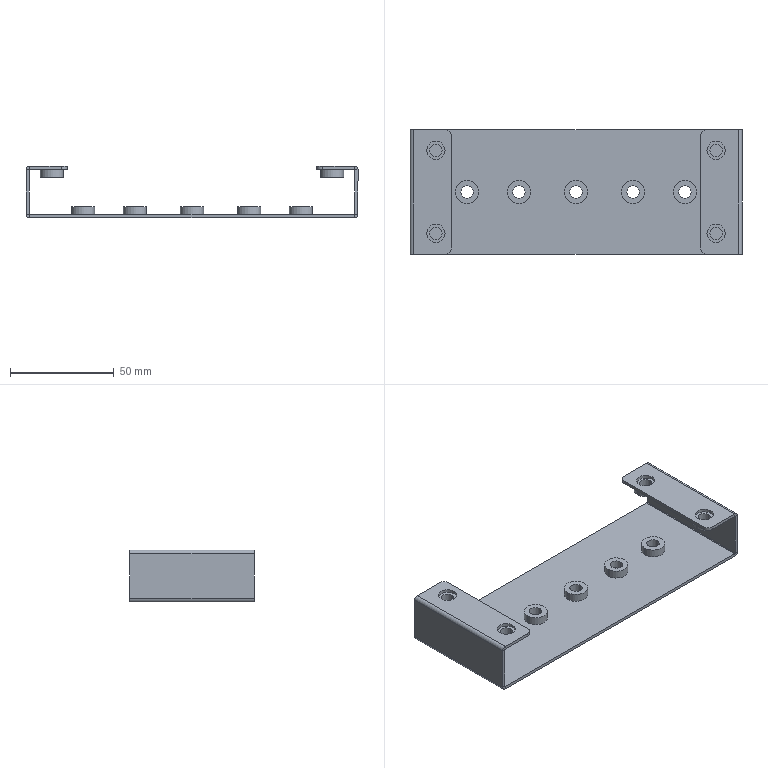Part | STEP file | FBDS-BJ-016 | 1 solid | 114 faces | box 160 x 60 x 25 mm | volume 23506 mm3 | cylinder 66 | plane 48 | commonest cylinder face diameters 6 x22 8.75 x18 11.18 x18 0.4 x4 3.4 x4